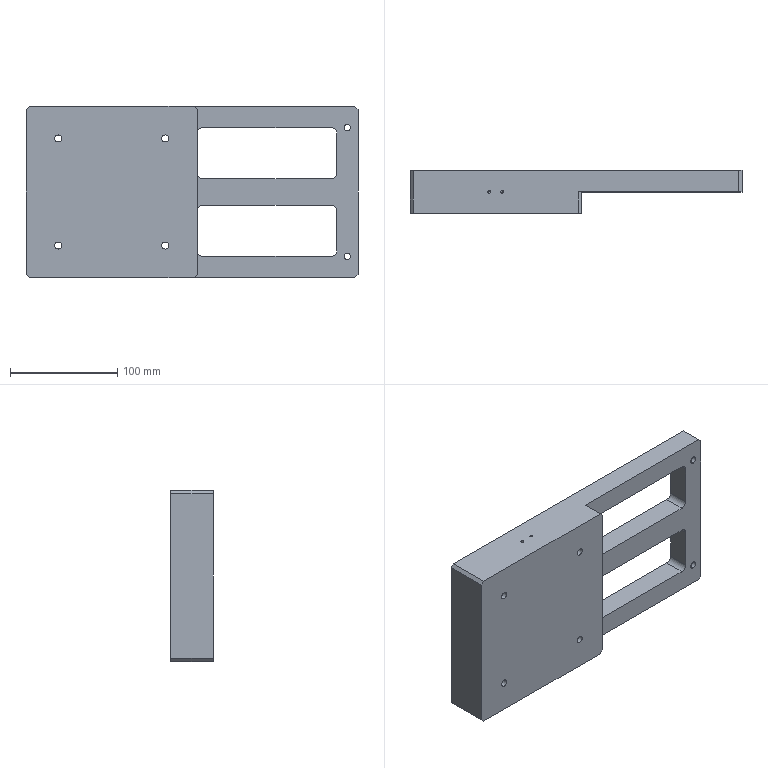CAM job | NX | 3+2 milling, drilling | part box 310 x 40 x 160 mm | stock box 315 x 45 x 165 mm
Tools:
number,name,description,diameter,corner_radius,flute_length,length,flutes
4,D4,平底铣刀-粗,4.0,0.0,25.0,75.0,2
6,D6,平底铣刀-粗,6.0,0.0,25.0,75.0,2
9,D10,平底铣刀-粗,10.0,0.0,35.0,75.0,2
11,D4-J,平底铣刀-精,4.0,0.0,50.0,75.0,2
7,D6-J,平底铣刀-精,6.0,0.0,25.0,75.0,2
10,D10-J,平底铣刀-精,10.0,0.0,35.0,75.0,2
1,D80R0.8飞刀,圆鼻刀-粗,80.0,0.8,50.0,75.0,2
1,D80R0.8飞刀-J,圆鼻刀-精,80.0,0.8,50.0,75.0,2
2,D6倒角刀,倒角刀,6.0,0.0,3.0,25.0,2
19,M8X1.25,丝锥,6.8,0.0,35.0,50.0,2
17,ZT5.8,钻头,5.8,0.0,35.0,50.0,2
18,ZT6.6,钻头,6.6,0.0,35.0,50.0,2
16,ZT6.8,钻头,6.8,0.0,35.0,50.0,2
Operations:
program,operation,operation_type,tool,method,geometry_group,spindle_rpm,surface_speed,feed_per_tooth,feed_cut,feed_plunge,cut_length_mm,path_length_mm,cut_time_min,machine_time_min
B,底壁铣飞面开粗_COPY,VolumeBased25DMillingOperation,D80R0.8飞刀,分层开粗-切深K-步距G,W-B,2800.0,703.696,0.5357,3000.0,100.0,11607.128,15223.834,3.869,4.231
B,底壁铣飞面精光_COPY,VolumeBased25DMillingOperation,D80R0.8飞刀-J,侧刃精光-切深K-步距G,W-B,4000.0,1005.28,0.125,1000.0,100.0,1289.241,1325.241,1.289,1.293
B,底壁铣分层开粗-中_COPY,VolumeBased25DMillingOperation,D10,分层开粗-切深K-步距G,W-B,8000.0,251.327,0.3125,5000.0,100.0,126568.912,135918.509,25.314,26.249
B,平面去毛刺6X45L_COPY,SurfaceContour,D6倒角刀,爬面_倒角-切深0-步距G,W-B,6500.0,122.519,0.1154,1500.0,100.0,1911.811,3163.014,1.274,1.4
B,底壁铣精光底面-中_COPY,VolumeBased25DMillingOperation,D6-J,精光步距切深关,W-B,6000.0,113.097,0.0833,1000.0,100.0,4476.68,4795.984,4.477,4.509
B,等高精光-中_COPY_1,ZLevelMilling,D6-J,侧刃精光-切深K-步距G,W-B,6000.0,113.097,0.0833,1000.0,100.0,688.868,1357.707,0.6889,0.7558
A,顶面,FaceMilling,D80R0.8飞刀,侧刃精光-切深K-步距G,W-A,4000.0,1005.31,0.125,1000.0,100.0,1718.0,1754.0,1.718,1.722
A,外形粗_2,VolumeBased25DMillingOperation,D10,METHOD,W-A,8000.0,251.327,0.3125,5000.0,80.0,51147.301,51226.101,10.229,10.237
A,型腔铣开粗-中_COPY,CavityMilling,D10,分层开粗-切深K-步距G,W-A,8000.0,251.32,0.25,4000.0,100.0,76853.678,78751.629,19.213,19.494
A,打点-深0.8,Operation,D6倒角刀,NONE,W-A,8000.0,150.796,0.0312,500.0,90.0,18.0,733.959,0.036,0.1076
A,通孔-精孔6.0预钻14.8,Operation,ZT5.8,NONE,W-A,2500.0,45.553,0.03,150.0,90.0,19.405,369.812,0.1294,0.1644
A,沉头孔-钻孔0段,Operation,ZT6.6,NONE,W-A,1200.0,24.881,0.0625,150.0,90.0,179.931,702.878,1.2,1.252
A,盲锥孔-M8螺纹底孔,Operation,ZT6.8,NONE,W-A,2200.0,46.998,0.0341,150.0,90.0,52.0,265.004,0.3467,0.368
A,通孔-M8螺纹底孔,Operation,ZT6.8,NONE,W-A,1800.0,38.453,0.0972,350.0,90.0,52.0,265.004,0.1486,0.1699
A,铣孔开粗D6_1,CylinderMilling,D6,NONE,W-A,8000.0,150.796,0.075,1200.0,100.0,3168.416,3726.416,2.64,2.696
A,铣孔精光D6_1,CylinderMilling,D6-J,精光步距切深关,W-A,8000.0,150.796,0.0312,500.0,100.0,423.751,983.751,0.8475,0.9035
A,铣孔开粗D4_1,CylinderMilling,D4,NONE,W-A,8000.0,100.531,0.0375,600.0,100.0,313.409,696.409,0.5223,0.5606
A,仅选体,SurfaceContour,D6倒角刀,METHOD,W-A,8000.0,150.796,0.1875,3000.0,100.0,1645.061,1878.604,0.5484,0.5717
A,铣倒角_1,PlanarMilling,D6倒角刀,METHOD,W-A,8000.0,150.796,0.0312,500.0,100.0,41.927,411.633,0.0839,0.1208
A,铣倒角_2,PlanarMilling,D6倒角刀,METHOD,W-A,8000.0,150.796,0.0375,600.0,100.0,62.549,265.415,0.1042,0.1245
A,铣倒角_3,PlanarMilling,D6倒角刀,METHOD,W-A,8000.0,150.796,0.0375,600.0,100.0,48.803,252.44,0.0813,0.1017
A,铣倒角_4,PlanarMilling,D6倒角刀,NONE,W-A,8000.0,150.796,0.05,800.0,100.0,173.57,611.374,0.217,0.2607
A,盲平孔-攻牙M8,Operation,M8X1.25,METHOD,W-A,500.0,10.681,0.0013,1.25,90.0,84.0,741.01,67.2,67.266
A,铣孔精光D4-J_1,CylinderMilling,D4-J,精光步距切深关,W-A,8000.0,100.531,0.0125,200.0,100.0,115.195,498.195,0.576,0.6143
A,等高精光-中_COPY,ZLevelMilling,D6-J,侧刃精光-切深K-步距G,W-A,8000.0,150.792,0.0625,1000.0,100.0,2666.091,2931.744,2.666,2.693
A,外形半精_2,VolumeBased25DMillingOperation,D10-J,METHOD,W-A,8000.0,251.327,0.0625,1000.0,100.0,2908.034,3191.263,2.908,2.936